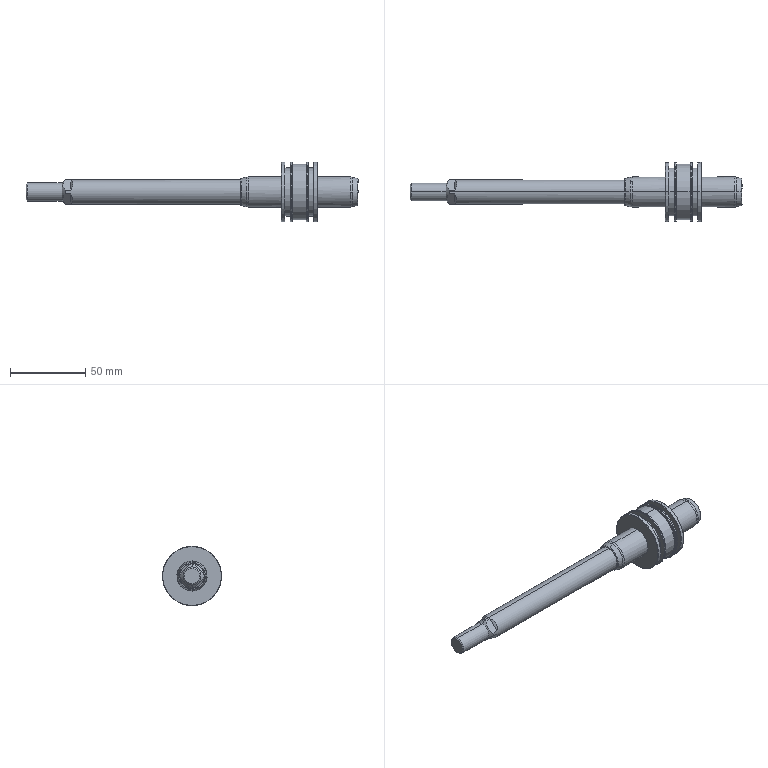Part | STEP file | SI-40X75-S-B1N-2-2 | 1 solid | 82 faces | box 220.5 x 39.5 x 39.5 mm | volume 58608 mm3 | cone 26 | cylinder 24 | plane 20 | spline 10 | other 2 | commonest cylinder face diameters 39.5 x8 20 x4 32 x4 12 x2 16 x2 16.5 x2